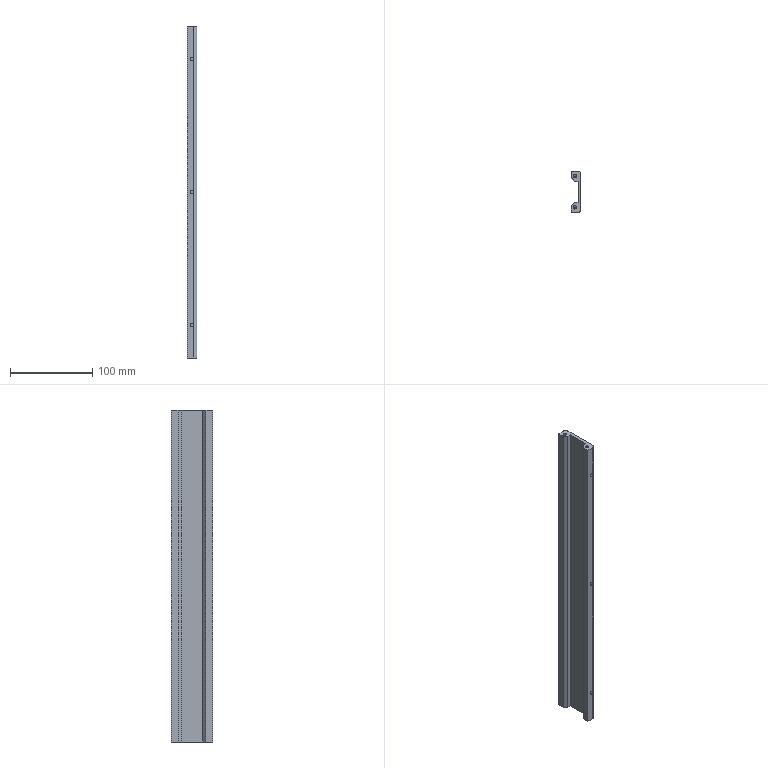Part | STEP file | PN_0016 | 1 solid | 36 faces | box 12 x 50 x 404 mm | volume 142558 mm3 | cylinder 16 | plane 12 | cone 8 | commonest cylinder face diameters 4.2 x14 8 x2